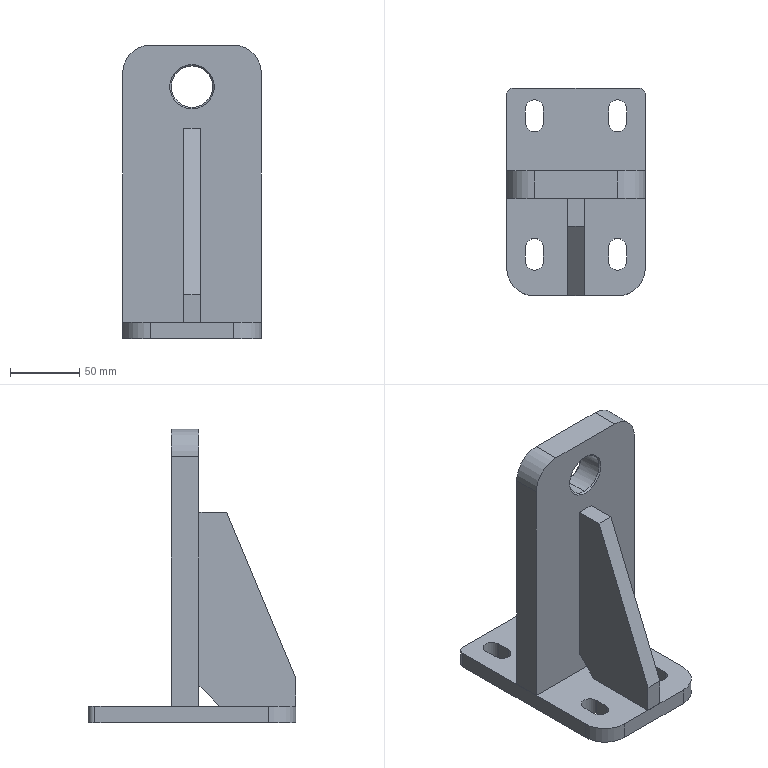Part | STEP file | 3 solids | 48 faces | box 100 x 150 x 212 mm | volume 627783 mm3 | plane 28 | cylinder 16 | cone 4 | commonest cylinder face diameters 13 x8 40 x4 10 x2 30 x2